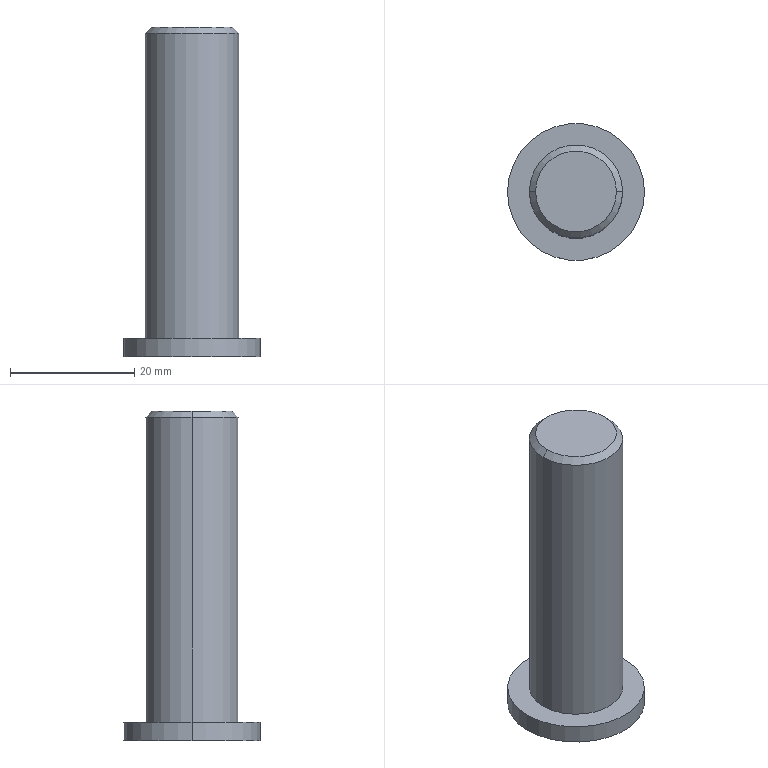Part | SolidWorks | features Chamfer 1, Extrusion 1, ICE 1 | 1 solid | 9 faces | box 22 x 22 x 53 mm | volume 9954 mm3 | cylinder 4 | plane 3 | cone 2 | commonest cylinder face diameters 15 x2 22 x2
STEP:
#1=CARTESIAN_POINT('',(6.5,0.,53.));
#2=VERTEX_POINT('',#1);
#3=CARTESIAN_POINT('',(-6.5,0.,53.));
#4=VERTEX_POINT('',#3);
#5=CARTESIAN_POINT('',(0.,0.,53.));
#6=DIRECTION('',(0.,0.,1.));
#7=DIRECTION('',(1.,0.,0.));
#8=AXIS2_PLACEMENT_3D('',#5,#6,#7);
#9=CIRCLE('',#8,6.5);
#10=EDGE_CURVE('',#2,#4,#9,.T.);
#11=ORIENTED_EDGE('',*,*,#10,.F.);
#12=CARTESIAN_POINT('',(7.5,0.,52.));
#13=VERTEX_POINT('',#12);
#14=CARTESIAN_POINT('',(6.5,0.,53.));
#15=DIRECTION('',(0.7071,0.,-0.7071));
#16=VECTOR('',#15,1000.);
#17=LINE('',#14,#16);
#18=EDGE_CURVE('',#2,#13,#17,.T.);
#19=ORIENTED_EDGE('',*,*,#18,.T.);
#20=CARTESIAN_POINT('',(-7.5,0.,52.));
#21=VERTEX_POINT('',#20);
#22=CARTESIAN_POINT('',(0.,0.,52.));
#23=DIRECTION('',(0.,0.,-1.));
#24=DIRECTION('',(1.,0.,0.));
#25=AXIS2_PLACEMENT_3D('',#22,#23,#24);
#26=CIRCLE('',#25,7.5);
#27=EDGE_CURVE('',#21,#13,#26,.T.);
#28=ORIENTED_EDGE('',*,*,#27,.F.);
#29=CARTESIAN_POINT('',(-6.5,0.,53.));
#30=DIRECTION('',(-0.7071,0.,-0.7071));
#31=VECTOR('',#30,1000.);
#32=LINE('',#29,#31);
#33=EDGE_CURVE('',#4,#21,#32,.T.);
#34=ORIENTED_EDGE('',*,*,#33,.F.);
#35=EDGE_LOOP('',(#11,#19,#28,#34));
#36=FACE_OUTER_BOUND('',#35,.T.);
#37=CARTESIAN_POINT('',(0.,0.,53.));
#38=DIRECTION('',(0.,0.,-1.));
#39=DIRECTION('',(-1.,0.,0.));
#40=AXIS2_PLACEMENT_3D('',#37,#38,#39);
#41=CONICAL_SURFACE('',#40,6.5,0.7854);
#42=ADVANCED_FACE('',(#36),#41,.T.);
#43=ORIENTED_EDGE('',*,*,#27,.T.);
#44=CARTESIAN_POINT('',(7.5,0.,3.));
#45=VERTEX_POINT('',#44);
#46=CARTESIAN_POINT('',(7.5,0.,53.));
#47=DIRECTION('',(0.,0.,-1.));
#48=VECTOR('',#47,1000.);
#49=LINE('',#46,#48);
#50=EDGE_CURVE('',#13,#45,#49,.T.);
#51=ORIENTED_EDGE('',*,*,#50,.T.);
#52=CARTESIAN_POINT('',(-7.5,0.,3.));
#53=VERTEX_POINT('',#52);
#54=CARTESIAN_POINT('',(0.,0.,3.));
#55=DIRECTION('',(0.,0.,1.));
#56=DIRECTION('',(1.,0.,0.));
#57=AXIS2_PLACEMENT_3D('',#54,#55,#56);
#58=CIRCLE('',#57,7.5);
#59=EDGE_CURVE('',#45,#53,#58,.T.);
#60=ORIENTED_EDGE('',*,*,#59,.T.);
#61=CARTESIAN_POINT('',(-7.5,0.,53.));
#62=DIRECTION('',(0.,0.,-1.));
#63=VECTOR('',#62,1000.);
#64=LINE('',#61,#63);
#65=EDGE_CURVE('',#21,#53,#64,.T.);
#66=ORIENTED_EDGE('',*,*,#65,.F.);
#67=EDGE_LOOP('',(#43,#51,#60,#66));
#68=FACE_OUTER_BOUND('',#67,.T.);
#69=CARTESIAN_POINT('',(0.,0.,53.));
#70=DIRECTION('',(0.,0.,-1.));
#71=DIRECTION('',(-1.,0.,0.));
#72=AXIS2_PLACEMENT_3D('',#69,#70,#71);
#73=CYLINDRICAL_SURFACE('',#72,7.5);
#74=ADVANCED_FACE('',(#68),#73,.T.);
#75=CARTESIAN_POINT('',(11.,0.,3.));
#76=VERTEX_POINT('',#75);
#77=CARTESIAN_POINT('',(-11.,0.,3.));
#78=VERTEX_POINT('',#77);
#79=CARTESIAN_POINT('',(0.,0.,3.));
#80=DIRECTION('',(0.,0.,1.));
#81=DIRECTION('',(1.,0.,0.));
#82=AXIS2_PLACEMENT_3D('',#79,#80,#81);
#83=CIRCLE('',#82,11.);
#84=EDGE_CURVE('',#76,#78,#83,.T.);
#85=ORIENTED_EDGE('',*,*,#84,.F.);
#86=CARTESIAN_POINT('',(11.,0.,0.));
#87=VERTEX_POINT('',#86);
#88=CARTESIAN_POINT('',(11.,0.,3.));
#89=DIRECTION('',(0.,0.,-1.));
#90=VECTOR('',#89,1000.);
#91=LINE('',#88,#90);
#92=EDGE_CURVE('',#76,#87,#91,.T.);
#93=ORIENTED_EDGE('',*,*,#92,.T.);
#94=CARTESIAN_POINT('',(-11.,0.,0.));
#95=VERTEX_POINT('',#94);
#96=CARTESIAN_POINT('',(0.,0.,0.));
#97=DIRECTION('',(0.,0.,1.));
#98=DIRECTION('',(1.,0.,0.));
#99=AXIS2_PLACEMENT_3D('',#96,#97,#98);
#100=CIRCLE('',#99,11.);
#101=EDGE_CURVE('',#87,#95,#100,.T.);
#102=ORIENTED_EDGE('',*,*,#101,.T.);
#103=CARTESIAN_POINT('',(-11.,0.,3.));
#104=DIRECTION('',(0.,0.,-1.));
#105=VECTOR('',#104,1000.);
#106=LINE('',#103,#105);
#107=EDGE_CURVE('',#78,#95,#106,.T.);
#108=ORIENTED_EDGE('',*,*,#107,.F.);
#109=EDGE_LOOP('',(#85,#93,#102,#108));
#110=FACE_OUTER_BOUND('',#109,.T.);
#111=CARTESIAN_POINT('',(0.,0.,3.));
#112=DIRECTION('',(0.,0.,-1.));
#113=DIRECTION('',(-1.,0.,0.));
#114=AXIS2_PLACEMENT_3D('',#111,#112,#113);
#115=CYLINDRICAL_SURFACE('',#114,11.);
#116=ADVANCED_FACE('',(#110),#115,.T.);
#117=ORIENTED_EDGE('',*,*,#92,.F.);
#118=CARTESIAN_POINT('',(0.,0.,3.));
#119=DIRECTION('',(0.,0.,1.));
#120=DIRECTION('',(1.,0.,0.));
#121=AXIS2_PLACEMENT_3D('',#118,#119,#120);
#122=CIRCLE('',#121,11.);
#123=EDGE_CURVE('',#78,#76,#122,.T.);
#124=ORIENTED_EDGE('',*,*,#123,.F.);
#125=ORIENTED_EDGE('',*,*,#107,.T.);
#126=CARTESIAN_POINT('',(0.,0.,0.));
#127=DIRECTION('',(0.,0.,1.));
#128=DIRECTION('',(1.,0.,0.));
#129=AXIS2_PLACEMENT_3D('',#126,#127,#128);
#130=CIRCLE('',#129,11.);
#131=EDGE_CURVE('',#95,#87,#130,.T.);
#132=ORIENTED_EDGE('',*,*,#131,.T.);
#133=EDGE_LOOP('',(#117,#124,#125,#132));
#134=FACE_OUTER_BOUND('',#133,.T.);
#135=CARTESIAN_POINT('',(0.,0.,3.));
#136=DIRECTION('',(0.,0.,-1.));
#137=DIRECTION('',(-1.,0.,0.));
#138=AXIS2_PLACEMENT_3D('',#135,#136,#137);
#139=CYLINDRICAL_SURFACE('',#138,11.);
#140=ADVANCED_FACE('',(#134),#139,.T.);
#141=CARTESIAN_POINT('',(0.,0.,3.));
#142=DIRECTION('',(0.,0.,1.));
#143=DIRECTION('',(1.,0.,0.));
#144=AXIS2_PLACEMENT_3D('',#141,#142,#143);
#145=CIRCLE('',#144,7.5);
#146=EDGE_CURVE('',#53,#45,#145,.T.);
#147=ORIENTED_EDGE('',*,*,#146,.F.);
#148=ORIENTED_EDGE('',*,*,#59,.F.);
#149=EDGE_LOOP('',(#147,#148));
#150=FACE_BOUND('',#149,.T.);
#151=ORIENTED_EDGE('',*,*,#123,.T.);
#152=ORIENTED_EDGE('',*,*,#84,.T.);
#153=EDGE_LOOP('',(#151,#152));
#154=FACE_OUTER_BOUND('',#153,.T.);
#155=CARTESIAN_POINT('',(0.,0.,3.));
#156=DIRECTION('',(0.,0.,1.));
#157=DIRECTION('',(1.,0.,0.));
#158=AXIS2_PLACEMENT_3D('',#155,#156,#157);
#159=PLANE('',#158);
#160=ADVANCED_FACE('',(#150,#154),#159,.T.);
#161=ORIENTED_EDGE('',*,*,#131,.F.);
#162=ORIENTED_EDGE('',*,*,#101,.F.);
#163=EDGE_LOOP('',(#161,#162));
#164=FACE_OUTER_BOUND('',#163,.T.);
#165=CARTESIAN_POINT('',(0.,0.,0.));
#166=DIRECTION('',(0.,0.,1.));
#167=DIRECTION('',(1.,0.,0.));
#168=AXIS2_PLACEMENT_3D('',#165,#166,#167);
#169=PLANE('',#168);
#170=ADVANCED_FACE('',(#164),#169,.F.);
#171=ORIENTED_EDGE('',*,*,#50,.F.);
#172=CARTESIAN_POINT('',(0.,0.,52.));
#173=DIRECTION('',(0.,0.,-1.));
#174=DIRECTION('',(1.,0.,0.));
#175=AXIS2_PLACEMENT_3D('',#172,#173,#174);
#176=CIRCLE('',#175,7.5);
#177=EDGE_CURVE('',#13,#21,#176,.T.);
#178=ORIENTED_EDGE('',*,*,#177,.T.);
#179=ORIENTED_EDGE('',*,*,#65,.T.);
#180=ORIENTED_EDGE('',*,*,#146,.T.);
#181=EDGE_LOOP('',(#171,#178,#179,#180));
#182=FACE_OUTER_BOUND('',#181,.T.);
#183=CARTESIAN_POINT('',(0.,0.,53.));
#184=DIRECTION('',(0.,0.,-1.));
#185=DIRECTION('',(-1.,0.,0.));
#186=AXIS2_PLACEMENT_3D('',#183,#184,#185);
#187=CYLINDRICAL_SURFACE('',#186,7.5);
#188=ADVANCED_FACE('',(#182),#187,.T.);
#189=CARTESIAN_POINT('',(0.,0.,53.));
#190=DIRECTION('',(0.,0.,1.));
#191=DIRECTION('',(1.,0.,0.));
#192=AXIS2_PLACEMENT_3D('',#189,#190,#191);
#193=CIRCLE('',#192,6.5);
#194=EDGE_CURVE('',#4,#2,#193,.T.);
#195=ORIENTED_EDGE('',*,*,#194,.T.);
#196=ORIENTED_EDGE('',*,*,#10,.T.);
#197=EDGE_LOOP('',(#195,#196));
#198=FACE_OUTER_BOUND('',#197,.T.);
#199=CARTESIAN_POINT('',(0.,0.,53.));
#200=DIRECTION('',(0.,0.,1.));
#201=DIRECTION('',(1.,0.,0.));
#202=AXIS2_PLACEMENT_3D('',#199,#200,#201);
#203=PLANE('',#202);
#204=ADVANCED_FACE('',(#198),#203,.T.);
#205=ORIENTED_EDGE('',*,*,#18,.F.);
#206=ORIENTED_EDGE('',*,*,#194,.F.);
#207=ORIENTED_EDGE('',*,*,#33,.T.);
#208=ORIENTED_EDGE('',*,*,#177,.F.);
#209=EDGE_LOOP('',(#205,#206,#207,#208));
#210=FACE_OUTER_BOUND('',#209,.T.);
#211=CARTESIAN_POINT('',(0.,0.,53.));
#212=DIRECTION('',(0.,0.,-1.));
#213=DIRECTION('',(-1.,0.,0.));
#214=AXIS2_PLACEMENT_3D('',#211,#212,#213);
#215=CONICAL_SURFACE('',#214,6.5,0.7854);
#216=ADVANCED_FACE('',(#210),#215,.T.);
#217=CLOSED_SHELL('',(#42,#74,#116,#140,#160,#170,#188,#204,#216));
#218=MANIFOLD_SOLID_BREP('',#217);
#219=CARTESIAN_POINT('',(0.,0.,0.));
#220=DIRECTION('',(0.,0.,1.));
#221=DIRECTION('',(1.,0.,0.));
#222=AXIS2_PLACEMENT_3D('',#219,#220,#221);
#223=(LENGTH_UNIT()NAMED_UNIT(*)SI_UNIT(.MILLI.,.METRE.));
#224=UNCERTAINTY_MEASURE_WITH_UNIT(LENGTH_MEASURE(0.00001),#223,'','');
#225=(NAMED_UNIT(*)PLANE_ANGLE_UNIT()SI_UNIT($,.RADIAN.));
#226=(NAMED_UNIT(*)SI_UNIT($,.STERADIAN.)SOLID_ANGLE_UNIT());
#227=(GEOMETRIC_REPRESENTATION_CONTEXT(3)GLOBAL_UNCERTAINTY_ASSIGNED_CONTEXT((#224))GLOBAL_UNIT_ASSIGNED_CONTEXT((#223,#225,#226))REPRESENTATION_CONTEXT('',''));
#228=ADVANCED_BREP_SHAPE_REPRESENTATION('',(#218,#222),#227);